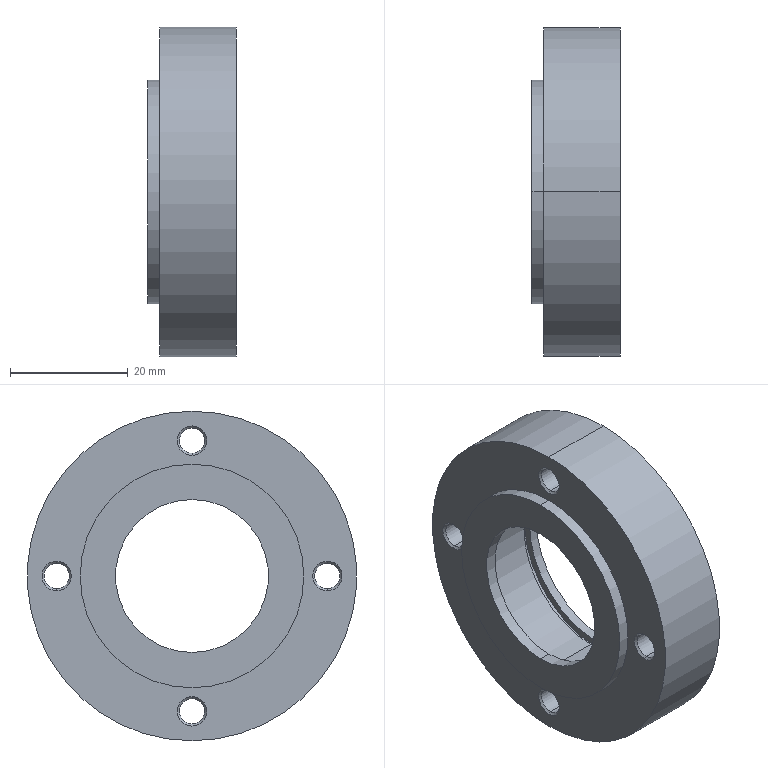Part | STEP file | Bearing seat BARR6201DD_b V1.201001 | 1 solid | 54 faces | box 15 x 56 x 56 mm | volume 21210 mm3 | cylinder 28 | cone 16 | plane 10 | commonest cylinder face diameters 4.3 x8 8 x8 32 x4 26 x2 34.4 x2 38 x2